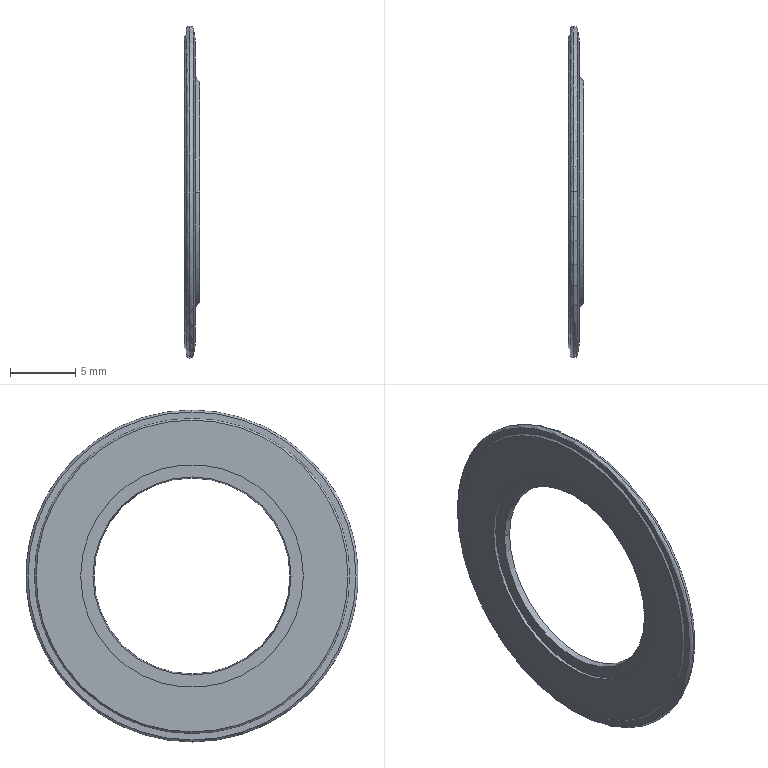Part | SolidWorks | features BaseBody 1 | 1 solid | 23 faces | box 1.155 x 25.353 x 25.353 mm | volume 176.021 mm3 | cone 8 | cylinder 6 | plane 5 | torus 4 | commonest cylinder face diameters 17 x4 23.324 x2
STEP:
#1=CARTESIAN_POINT('',(0.456,0.,12.676));
#2=VERTEX_POINT('',#1);
#3=CARTESIAN_POINT('',(0.456,0.,-12.676));
#4=VERTEX_POINT('',#3);
#5=CARTESIAN_POINT('',(0.456,0.,0.));
#6=DIRECTION('',(1.,0.,0.));
#7=DIRECTION('',(0.,0.,-1.));
#8=AXIS2_PLACEMENT_3D('',#5,#6,#7);
#9=CIRCLE('',#8,12.676);
#10=EDGE_CURVE('',#2,#4,#9,.T.);
#11=ORIENTED_EDGE('',*,*,#10,.T.);
#12=CARTESIAN_POINT('',(0.7554,0.,-12.425));
#13=VERTEX_POINT('',#12);
#14=CARTESIAN_POINT('',(0.456,0.,-12.372));
#15=DIRECTION('',(0.,-1.,0.));
#16=DIRECTION('',(0.,0.,-1.));
#17=AXIS2_PLACEMENT_3D('',#14,#15,#16);
#18=CIRCLE('',#17,0.304);
#19=EDGE_CURVE('',#4,#13,#18,.T.);
#20=ORIENTED_EDGE('',*,*,#19,.T.);
#21=CARTESIAN_POINT('',(0.7554,-12.425,0.));
#22=VERTEX_POINT('',#21);
#23=CARTESIAN_POINT('',(0.7554,0.,0.));
#24=DIRECTION('',(1.,0.,0.));
#25=DIRECTION('',(0.,1.,0.));
#26=AXIS2_PLACEMENT_3D('',#23,#24,#25);
#27=CIRCLE('',#26,12.425);
#28=EDGE_CURVE('',#22,#13,#27,.T.);
#29=ORIENTED_EDGE('',*,*,#28,.F.);
#30=CARTESIAN_POINT('',(0.7554,0.,12.425));
#31=VERTEX_POINT('',#30);
#32=CARTESIAN_POINT('',(0.7554,0.,0.));
#33=DIRECTION('',(1.,0.,0.));
#34=DIRECTION('',(0.,1.,0.));
#35=AXIS2_PLACEMENT_3D('',#32,#33,#34);
#36=CIRCLE('',#35,12.425);
#37=EDGE_CURVE('',#31,#22,#36,.T.);
#38=ORIENTED_EDGE('',*,*,#37,.F.);
#39=CARTESIAN_POINT('',(0.456,0.,12.372));
#40=DIRECTION('',(0.,-1.,0.));
#41=DIRECTION('',(0.,0.,1.));
#42=AXIS2_PLACEMENT_3D('',#39,#40,#41);
#43=CIRCLE('',#42,0.304);
#44=EDGE_CURVE('',#31,#2,#43,.T.);
#45=ORIENTED_EDGE('',*,*,#44,.T.);
#46=EDGE_LOOP('',(#11,#20,#29,#38,#45));
#47=FACE_OUTER_BOUND('',#46,.T.);
#48=CARTESIAN_POINT('',(0.456,0.,0.));
#49=DIRECTION('',(1.,0.,0.));
#50=DIRECTION('',(0.,0.,-1.));
#51=AXIS2_PLACEMENT_3D('',#48,#49,#50);
#52=TOROIDAL_SURFACE('',#51,12.372,0.304);
#53=ADVANCED_FACE('',(#47),#52,.T.);
#54=CARTESIAN_POINT('',(0.1927,12.038,0.));
#55=VERTEX_POINT('',#54);
#56=CARTESIAN_POINT('',(0.1927,-12.038,0.));
#57=VERTEX_POINT('',#56);
#58=CARTESIAN_POINT('',(0.1927,0.,0.));
#59=DIRECTION('',(1.,0.,0.));
#60=DIRECTION('',(0.,1.,0.));
#61=AXIS2_PLACEMENT_3D('',#58,#59,#60);
#62=CIRCLE('',#61,12.038);
#63=EDGE_CURVE('',#55,#57,#62,.T.);
#64=ORIENTED_EDGE('',*,*,#63,.T.);
#65=CARTESIAN_POINT('',(0.1927,0.,0.));
#66=DIRECTION('',(1.,0.,0.));
#67=DIRECTION('',(0.,1.,0.));
#68=AXIS2_PLACEMENT_3D('',#65,#66,#67);
#69=CIRCLE('',#68,12.038);
#70=EDGE_CURVE('',#57,#55,#69,.T.);
#71=ORIENTED_EDGE('',*,*,#70,.T.);
#72=EDGE_LOOP('',(#64,#71));
#73=FACE_BOUND('',#72,.T.);
#74=CARTESIAN_POINT('',(0.1927,0.,-12.524));
#75=VERTEX_POINT('',#74);
#76=CARTESIAN_POINT('',(0.1927,0.,12.524));
#77=VERTEX_POINT('',#76);
#78=CARTESIAN_POINT('',(0.1927,0.,0.));
#79=DIRECTION('',(1.,0.,0.));
#80=DIRECTION('',(0.,1.,0.));
#81=AXIS2_PLACEMENT_3D('',#78,#79,#80);
#82=CIRCLE('',#81,12.524);
#83=EDGE_CURVE('',#75,#77,#82,.T.);
#84=ORIENTED_EDGE('',*,*,#83,.F.);
#85=CARTESIAN_POINT('',(0.1927,0.,0.));
#86=DIRECTION('',(1.,0.,0.));
#87=DIRECTION('',(0.,1.,0.));
#88=AXIS2_PLACEMENT_3D('',#85,#86,#87);
#89=CIRCLE('',#88,12.524);
#90=EDGE_CURVE('',#77,#75,#89,.T.);
#91=ORIENTED_EDGE('',*,*,#90,.F.);
#92=EDGE_LOOP('',(#84,#91));
#93=FACE_OUTER_BOUND('',#92,.T.);
#94=CARTESIAN_POINT('',(0.1927,12.281,0.));
#95=DIRECTION('',(-1.,0.,0.));
#96=DIRECTION('',(0.,1.,0.));
#97=AXIS2_PLACEMENT_3D('',#94,#95,#96);
#98=PLANE('',#97);
#99=ADVANCED_FACE('',(#73,#93),#98,.T.);
#100=CARTESIAN_POINT('',(0.0608,11.906,0.));
#101=VERTEX_POINT('',#100);
#102=CARTESIAN_POINT('',(0.1268,11.972,0.));
#103=DIRECTION('',(0.7071,0.7071,0.));
#104=VECTOR('',#103,1000.);
#105=LINE('',#102,#104);
#106=EDGE_CURVE('',#101,#55,#105,.T.);
#107=ORIENTED_EDGE('',*,*,#106,.T.);
#108=ORIENTED_EDGE('',*,*,#70,.F.);
#109=CARTESIAN_POINT('',(0.0608,-11.906,0.));
#110=VERTEX_POINT('',#109);
#111=CARTESIAN_POINT('',(0.1268,-11.972,0.));
#112=DIRECTION('',(-0.7071,0.7071,0.));
#113=VECTOR('',#112,1000.);
#114=LINE('',#111,#113);
#115=EDGE_CURVE('',#57,#110,#114,.T.);
#116=ORIENTED_EDGE('',*,*,#115,.T.);
#117=CARTESIAN_POINT('',(0.0608,0.,0.));
#118=DIRECTION('',(1.,0.,0.));
#119=DIRECTION('',(0.,1.,0.));
#120=AXIS2_PLACEMENT_3D('',#117,#118,#119);
#121=CIRCLE('',#120,11.906);
#122=EDGE_CURVE('',#110,#101,#121,.T.);
#123=ORIENTED_EDGE('',*,*,#122,.T.);
#124=EDGE_LOOP('',(#107,#108,#116,#123));
#125=FACE_OUTER_BOUND('',#124,.T.);
#126=CARTESIAN_POINT('',(0.1268,0.,0.));
#127=DIRECTION('',(1.,0.,0.));
#128=DIRECTION('',(0.,1.,0.));
#129=AXIS2_PLACEMENT_3D('',#126,#127,#128);
#130=CONICAL_SURFACE('',#129,11.972,0.7854);
#131=ADVANCED_FACE('',(#125),#130,.T.);
#132=CARTESIAN_POINT('',(0.0608,8.5,0.));
#133=VERTEX_POINT('',#132);
#134=CARTESIAN_POINT('',(0.0608,-8.5,0.));
#135=VERTEX_POINT('',#134);
#136=CARTESIAN_POINT('',(0.0608,0.,0.));
#137=DIRECTION('',(1.,0.,0.));
#138=DIRECTION('',(0.,1.,0.));
#139=AXIS2_PLACEMENT_3D('',#136,#137,#138);
#140=CIRCLE('',#139,8.5);
#141=EDGE_CURVE('',#133,#135,#140,.T.);
#142=ORIENTED_EDGE('',*,*,#141,.T.);
#143=CARTESIAN_POINT('',(0.0608,0.,0.));
#144=DIRECTION('',(1.,0.,0.));
#145=DIRECTION('',(0.,1.,0.));
#146=AXIS2_PLACEMENT_3D('',#143,#144,#145);
#147=CIRCLE('',#146,8.5);
#148=EDGE_CURVE('',#135,#133,#147,.T.);
#149=ORIENTED_EDGE('',*,*,#148,.T.);
#150=EDGE_LOOP('',(#142,#149));
#151=FACE_BOUND('',#150,.T.);
#152=CARTESIAN_POINT('',(0.0608,0.,0.));
#153=DIRECTION('',(1.,0.,0.));
#154=DIRECTION('',(0.,1.,0.));
#155=AXIS2_PLACEMENT_3D('',#152,#153,#154);
#156=CIRCLE('',#155,11.906);
#157=EDGE_CURVE('',#101,#110,#156,.T.);
#158=ORIENTED_EDGE('',*,*,#157,.F.);
#159=ORIENTED_EDGE('',*,*,#122,.F.);
#160=EDGE_LOOP('',(#158,#159));
#161=FACE_OUTER_BOUND('',#160,.T.);
#162=CARTESIAN_POINT('',(0.0608,10.203,0.));
#163=DIRECTION('',(-1.,0.,0.));
#164=DIRECTION('',(0.,0.,1.));
#165=AXIS2_PLACEMENT_3D('',#162,#163,#164);
#166=PLANE('',#165);
#167=ADVANCED_FACE('',(#151,#161),#166,.T.);
#168=CARTESIAN_POINT('',(0.2888,8.5,0.));
#169=VERTEX_POINT('',#168);
#170=CARTESIAN_POINT('',(0.1748,8.5,0.));
#171=DIRECTION('',(1.,0.,0.));
#172=VECTOR('',#171,1000.);
#173=LINE('',#170,#172);
#174=EDGE_CURVE('',#133,#169,#173,.T.);
#175=ORIENTED_EDGE('',*,*,#174,.T.);
#176=CARTESIAN_POINT('',(0.2888,-8.5,0.));
#177=VERTEX_POINT('',#176);
#178=CARTESIAN_POINT('',(0.2888,0.,0.));
#179=DIRECTION('',(1.,0.,0.));
#180=DIRECTION('',(0.,1.,0.));
#181=AXIS2_PLACEMENT_3D('',#178,#179,#180);
#182=CIRCLE('',#181,8.5);
#183=EDGE_CURVE('',#169,#177,#182,.T.);
#184=ORIENTED_EDGE('',*,*,#183,.T.);
#185=CARTESIAN_POINT('',(0.1748,-8.5,0.));
#186=DIRECTION('',(-1.,0.,0.));
#187=VECTOR('',#186,1000.);
#188=LINE('',#185,#187);
#189=EDGE_CURVE('',#177,#135,#188,.T.);
#190=ORIENTED_EDGE('',*,*,#189,.T.);
#191=ORIENTED_EDGE('',*,*,#141,.F.);
#192=EDGE_LOOP('',(#175,#184,#190,#191));
#193=FACE_OUTER_BOUND('',#192,.T.);
#194=CARTESIAN_POINT('',(0.1748,0.,0.));
#195=DIRECTION('',(1.,0.,0.));
#196=DIRECTION('',(0.,1.,0.));
#197=AXIS2_PLACEMENT_3D('',#194,#195,#196);
#198=CYLINDRICAL_SURFACE('',#197,8.5);
#199=ADVANCED_FACE('',(#193),#198,.F.);
#200=CARTESIAN_POINT('',(0.2888,7.565,0.));
#201=VERTEX_POINT('',#200);
#202=CARTESIAN_POINT('',(0.2888,-7.565,0.));
#203=VERTEX_POINT('',#202);
#204=CARTESIAN_POINT('',(0.2888,0.,0.));
#205=DIRECTION('',(1.,0.,0.));
#206=DIRECTION('',(0.,1.,0.));
#207=AXIS2_PLACEMENT_3D('',#204,#205,#206);
#208=CIRCLE('',#207,7.565);
#209=EDGE_CURVE('',#201,#203,#208,.T.);
#210=ORIENTED_EDGE('',*,*,#209,.T.);
#211=CARTESIAN_POINT('',(0.2888,0.,0.));
#212=DIRECTION('',(1.,0.,0.));
#213=DIRECTION('',(0.,1.,0.));
#214=AXIS2_PLACEMENT_3D('',#211,#212,#213);
#215=CIRCLE('',#214,7.565);
#216=EDGE_CURVE('',#203,#201,#215,.T.);
#217=ORIENTED_EDGE('',*,*,#216,.T.);
#218=EDGE_LOOP('',(#210,#217));
#219=FACE_BOUND('',#218,.T.);
#220=ORIENTED_EDGE('',*,*,#183,.F.);
#221=CARTESIAN_POINT('',(0.2888,0.,0.));
#222=DIRECTION('',(1.,0.,0.));
#223=DIRECTION('',(0.,1.,0.));
#224=AXIS2_PLACEMENT_3D('',#221,#222,#223);
#225=CIRCLE('',#224,8.5);
#226=EDGE_CURVE('',#177,#169,#225,.T.);
#227=ORIENTED_EDGE('',*,*,#226,.F.);
#228=EDGE_LOOP('',(#220,#227));
#229=FACE_OUTER_BOUND('',#228,.T.);
#230=CARTESIAN_POINT('',(0.2888,8.033,0.));
#231=DIRECTION('',(-1.,0.,0.));
#232=DIRECTION('',(0.,1.,0.));
#233=AXIS2_PLACEMENT_3D('',#230,#231,#232);
#234=PLANE('',#233);
#235=ADVANCED_FACE('',(#219,#229),#234,.T.);
#236=CARTESIAN_POINT('',(0.76,7.482,0.));
#237=VERTEX_POINT('',#236);
#238=CARTESIAN_POINT('',(0.5244,7.524,0.));
#239=DIRECTION('',(0.9848,-0.1736,0.));
#240=VECTOR('',#239,1000.);
#241=LINE('',#238,#240);
#242=EDGE_CURVE('',#201,#237,#241,.T.);
#243=ORIENTED_EDGE('',*,*,#242,.T.);
#244=CARTESIAN_POINT('',(0.76,-7.482,0.));
#245=VERTEX_POINT('',#244);
#246=CARTESIAN_POINT('',(0.76,0.,0.));
#247=DIRECTION('',(1.,0.,0.));
#248=DIRECTION('',(0.,1.,0.));
#249=AXIS2_PLACEMENT_3D('',#246,#247,#248);
#250=CIRCLE('',#249,7.482);
#251=EDGE_CURVE('',#237,#245,#250,.T.);
#252=ORIENTED_EDGE('',*,*,#251,.T.);
#253=CARTESIAN_POINT('',(0.5244,-7.524,0.));
#254=DIRECTION('',(-0.9848,-0.1736,0.));
#255=VECTOR('',#254,1000.);
#256=LINE('',#253,#255);
#257=EDGE_CURVE('',#245,#203,#256,.T.);
#258=ORIENTED_EDGE('',*,*,#257,.T.);
#259=ORIENTED_EDGE('',*,*,#209,.F.);
#260=EDGE_LOOP('',(#243,#252,#258,#259));
#261=FACE_OUTER_BOUND('',#260,.T.);
#262=CARTESIAN_POINT('',(0.5244,0.,0.));
#263=DIRECTION('',(-1.,0.,0.));
#264=DIRECTION('',(0.,1.,0.));
#265=AXIS2_PLACEMENT_3D('',#262,#263,#264);
#266=CONICAL_SURFACE('',#265,7.524,0.1745);
#267=ADVANCED_FACE('',(#261),#266,.F.);
#268=ORIENTED_EDGE('',*,*,#251,.F.);
#269=CARTESIAN_POINT('',(0.76,0.,0.));
#270=DIRECTION('',(1.,0.,0.));
#271=DIRECTION('',(0.,1.,0.));
#272=AXIS2_PLACEMENT_3D('',#269,#270,#271);
#273=CIRCLE('',#272,7.482);
#274=EDGE_CURVE('',#245,#237,#273,.T.);
#275=ORIENTED_EDGE('',*,*,#274,.F.);
#276=EDGE_LOOP('',(#268,#275));
#277=FACE_BOUND('',#276,.T.);
#278=CARTESIAN_POINT('',(0.76,8.5,0.));
#279=VERTEX_POINT('',#278);
#280=CARTESIAN_POINT('',(0.76,-8.5,0.));
#281=VERTEX_POINT('',#280);
#282=CARTESIAN_POINT('',(0.76,0.,0.));
#283=DIRECTION('',(1.,0.,0.));
#284=DIRECTION('',(0.,1.,0.));
#285=AXIS2_PLACEMENT_3D('',#282,#283,#284);
#286=CIRCLE('',#285,8.5);
#287=EDGE_CURVE('',#279,#281,#286,.T.);
#288=ORIENTED_EDGE('',*,*,#287,.T.);
#289=CARTESIAN_POINT('',(0.76,0.,0.));
#290=DIRECTION('',(1.,0.,0.));
#291=DIRECTION('',(0.,1.,0.));
#292=AXIS2_PLACEMENT_3D('',#289,#290,#291);
#293=CIRCLE('',#292,8.5);
#294=EDGE_CURVE('',#281,#279,#293,.T.);
#295=ORIENTED_EDGE('',*,*,#294,.T.);
#296=EDGE_LOOP('',(#288,#295));
#297=FACE_OUTER_BOUND('',#296,.T.);
#298=CARTESIAN_POINT('',(0.76,7.991,0.));
#299=DIRECTION('',(1.,0.,0.));
#300=DIRECTION('',(0.,1.,0.));
#301=AXIS2_PLACEMENT_3D('',#298,#299,#300);
#302=PLANE('',#301);
#303=ADVANCED_FACE('',(#277,#297),#302,.T.);
#304=CARTESIAN_POINT('',(1.216,8.5,0.));
#305=VERTEX_POINT('',#304);
#306=CARTESIAN_POINT('',(0.988,8.5,0.));
#307=DIRECTION('',(1.,0.,0.));
#308=VECTOR('',#307,1000.);
#309=LINE('',#306,#308);
#310=EDGE_CURVE('',#279,#305,#309,.T.);
#311=ORIENTED_EDGE('',*,*,#310,.T.);
#312=CARTESIAN_POINT('',(1.216,-8.5,0.));
#313=VERTEX_POINT('',#312);
#314=CARTESIAN_POINT('',(1.216,0.,0.));
#315=DIRECTION('',(1.,0.,0.));
#316=DIRECTION('',(0.,1.,0.));
#317=AXIS2_PLACEMENT_3D('',#314,#315,#316);
#318=CIRCLE('',#317,8.5);
#319=EDGE_CURVE('',#305,#313,#318,.T.);
#320=ORIENTED_EDGE('',*,*,#319,.T.);
#321=CARTESIAN_POINT('',(0.988,-8.5,0.));
#322=DIRECTION('',(-1.,0.,0.));
#323=VECTOR('',#322,1000.);
#324=LINE('',#321,#323);
#325=EDGE_CURVE('',#313,#281,#324,.T.);
#326=ORIENTED_EDGE('',*,*,#325,.T.);
#327=ORIENTED_EDGE('',*,*,#287,.F.);
#328=EDGE_LOOP('',(#311,#320,#326,#327));
#329=FACE_OUTER_BOUND('',#328,.T.);
#330=CARTESIAN_POINT('',(0.988,0.,0.));
#331=DIRECTION('',(1.,0.,0.));
#332=DIRECTION('',(0.,1.,0.));
#333=AXIS2_PLACEMENT_3D('',#330,#331,#332);
#334=CYLINDRICAL_SURFACE('',#333,8.5);
#335=ADVANCED_FACE('',(#329),#334,.F.);
#336=CARTESIAN_POINT('',(0.5168,9.199,0.));
#337=VERTEX_POINT('',#336);
#338=CARTESIAN_POINT('',(0.8664,8.85,0.));
#339=DIRECTION('',(0.7071,-0.7071,0.));
#340=VECTOR('',#339,1000.);
#341=LINE('',#338,#340);
#342=EDGE_CURVE('',#337,#305,#341,.T.);
#343=ORIENTED_EDGE('',*,*,#342,.T.);
#344=CARTESIAN_POINT('',(1.216,0.,0.));
#345=DIRECTION('',(1.,0.,0.));
#346=DIRECTION('',(0.,1.,0.));
#347=AXIS2_PLACEMENT_3D('',#344,#345,#346);
#348=CIRCLE('',#347,8.5);
#349=EDGE_CURVE('',#313,#305,#348,.T.);
#350=ORIENTED_EDGE('',*,*,#349,.F.);
#351=CARTESIAN_POINT('',(0.5168,-9.199,0.));
#352=VERTEX_POINT('',#351);
#353=CARTESIAN_POINT('',(0.8664,-8.85,0.));
#354=DIRECTION('',(-0.7071,-0.7071,0.));
#355=VECTOR('',#354,1000.);
#356=LINE('',#353,#355);
#357=EDGE_CURVE('',#313,#352,#356,.T.);
#358=ORIENTED_EDGE('',*,*,#357,.T.);
#359=CARTESIAN_POINT('',(0.5168,0.,0.));
#360=DIRECTION('',(1.,0.,0.));
#361=DIRECTION('',(0.,1.,0.));
#362=AXIS2_PLACEMENT_3D('',#359,#360,#361);
#363=CIRCLE('',#362,9.199);
#364=EDGE_CURVE('',#352,#337,#363,.T.);
#365=ORIENTED_EDGE('',*,*,#364,.T.);
#366=EDGE_LOOP('',(#343,#350,#358,#365));
#367=FACE_OUTER_BOUND('',#366,.T.);
#368=CARTESIAN_POINT('',(0.8664,0.,0.));
#369=DIRECTION('',(-1.,0.,0.));
#370=DIRECTION('',(0.,1.,0.));
#371=AXIS2_PLACEMENT_3D('',#368,#369,#370);
#372=CONICAL_SURFACE('',#371,8.85,0.7854);
#373=ADVANCED_FACE('',(#367),#372,.T.);
#374=CARTESIAN_POINT('',(0.5168,0.,0.));
#375=DIRECTION('',(1.,0.,0.));
#376=DIRECTION('',(0.,1.,0.));
#377=AXIS2_PLACEMENT_3D('',#374,#375,#376);
#378=CIRCLE('',#377,9.199);
#379=EDGE_CURVE('',#337,#352,#378,.T.);
#380=ORIENTED_EDGE('',*,*,#379,.F.);
#381=ORIENTED_EDGE('',*,*,#364,.F.);
#382=EDGE_LOOP('',(#380,#381));
#383=FACE_BOUND('',#382,.T.);
#384=CARTESIAN_POINT('',(0.5168,11.662,0.));
#385=VERTEX_POINT('',#384);
#386=CARTESIAN_POINT('',(0.5168,-11.662,0.));
#387=VERTEX_POINT('',#386);
#388=CARTESIAN_POINT('',(0.5168,0.,0.));
#389=DIRECTION('',(1.,0.,0.));
#390=DIRECTION('',(0.,1.,0.));
#391=AXIS2_PLACEMENT_3D('',#388,#389,#390);
#392=CIRCLE('',#391,11.662);
#393=EDGE_CURVE('',#385,#387,#392,.T.);
#394=ORIENTED_EDGE('',*,*,#393,.T.);
#395=CARTESIAN_POINT('',(0.5168,0.,0.));
#396=DIRECTION('',(1.,0.,0.));
#397=DIRECTION('',(0.,1.,0.));
#398=AXIS2_PLACEMENT_3D('',#395,#396,#397);
#399=CIRCLE('',#398,11.662);
#400=EDGE_CURVE('',#387,#385,#399,.T.);
#401=ORIENTED_EDGE('',*,*,#400,.T.);
#402=EDGE_LOOP('',(#394,#401));
#403=FACE_OUTER_BOUND('',#402,.T.);
#404=CARTESIAN_POINT('',(0.5168,10.431,0.));
#405=DIRECTION('',(1.,0.,0.));
#406=DIRECTION('',(0.,1.,0.));
#407=AXIS2_PLACEMENT_3D('',#404,#405,#406);
#408=PLANE('',#407);
#409=ADVANCED_FACE('',(#383,#403),#408,.T.);
#410=CARTESIAN_POINT('',(0.8899,11.662,0.));
#411=VERTEX_POINT('',#410);
#412=CARTESIAN_POINT('',(0.7034,11.662,0.));
#413=DIRECTION('',(1.,0.,0.));
#414=VECTOR('',#413,1000.);
#415=LINE('',#412,#414);
#416=EDGE_CURVE('',#385,#411,#415,.T.);
#417=ORIENTED_EDGE('',*,*,#416,.T.);
#418=CARTESIAN_POINT('',(0.8899,-11.662,0.));
#419=VERTEX_POINT('',#418);
#420=CARTESIAN_POINT('',(0.8899,0.,0.));
#421=DIRECTION('',(1.,0.,0.));
#422=DIRECTION('',(0.,1.,0.));
#423=AXIS2_PLACEMENT_3D('',#420,#421,#422);
#424=CIRCLE('',#423,11.662);
#425=EDGE_CURVE('',#411,#419,#424,.T.);
#426=ORIENTED_EDGE('',*,*,#425,.T.);
#427=CARTESIAN_POINT('',(0.7034,-11.662,0.));
#428=DIRECTION('',(-1.,0.,0.));
#429=VECTOR('',#428,1000.);
#430=LINE('',#427,#429);
#431=EDGE_CURVE('',#419,#387,#430,.T.);
#432=ORIENTED_EDGE('',*,*,#431,.T.);
#433=ORIENTED_EDGE('',*,*,#393,.F.);
#434=EDGE_LOOP('',(#417,#426,#432,#433));
#435=FACE_OUTER_BOUND('',#434,.T.);
#436=CARTESIAN_POINT('',(0.7034,0.,0.));
#437=DIRECTION('',(1.,0.,0.));
#438=DIRECTION('',(0.,1.,0.));
#439=AXIS2_PLACEMENT_3D('',#436,#437,#438);
#440=CYLINDRICAL_SURFACE('',#439,11.662);
#441=ADVANCED_FACE('',(#435),#440,.F.);
#442=CARTESIAN_POINT('',(0.7554,12.425,0.));
#443=VERTEX_POINT('',#442);
#444=CARTESIAN_POINT('',(0.8227,12.044,0.));
#445=DIRECTION('',(0.1736,-0.9848,0.));
#446=VECTOR('',#445,1000.);
#447=LINE('',#444,#446);
#448=EDGE_CURVE('',#443,#411,#447,.T.);
#449=ORIENTED_EDGE('',*,*,#448,.T.);
#450=CARTESIAN_POINT('',(0.8899,0.,0.));
#451=DIRECTION('',(1.,0.,0.));
#452=DIRECTION('',(0.,1.,0.));
#453=AXIS2_PLACEMENT_3D('',#450,#451,#452);
#454=CIRCLE('',#453,11.662);
#455=EDGE_CURVE('',#419,#411,#454,.T.);
#456=ORIENTED_EDGE('',*,*,#455,.F.);
#457=CARTESIAN_POINT('',(0.8227,-12.044,0.));
#458=DIRECTION('',(-0.1736,-0.9848,0.));
#459=VECTOR('',#458,1000.);
#460=LINE('',#457,#459);
#461=EDGE_CURVE('',#419,#22,#460,.T.);
#462=ORIENTED_EDGE('',*,*,#461,.T.);
#463=ORIENTED_EDGE('',*,*,#28,.T.);
#464=CARTESIAN_POINT('',(0.7554,0.,0.));
#465=DIRECTION('',(1.,0.,0.));
#466=DIRECTION('',(0.,1.,0.));
#467=AXIS2_PLACEMENT_3D('',#464,#465,#466);
#468=CIRCLE('',#467,12.425);
#469=EDGE_CURVE('',#13,#443,#468,.T.);
#470=ORIENTED_EDGE('',*,*,#469,.T.);
#471=EDGE_LOOP('',(#449,#456,#462,#463,#470));
#472=FACE_OUTER_BOUND('',#471,.T.);
#473=CARTESIAN_POINT('',(0.8227,0.,0.));
#474=DIRECTION('',(-1.,0.,0.));
#475=DIRECTION('',(0.,1.,0.));
#476=AXIS2_PLACEMENT_3D('',#473,#474,#475);
#477=CONICAL_SURFACE('',#476,12.044,1.396);
#478=ADVANCED_FACE('',(#472),#477,.T.);
#479=ORIENTED_EDGE('',*,*,#448,.F.);
#480=CARTESIAN_POINT('',(0.7554,0.,0.));
#481=DIRECTION('',(1.,0.,0.));
#482=DIRECTION('',(0.,1.,0.));
#483=AXIS2_PLACEMENT_3D('',#480,#481,#482);
#484=CIRCLE('',#483,12.425);
#485=EDGE_CURVE('',#443,#31,#484,.T.);
#486=ORIENTED_EDGE('',*,*,#485,.T.);
#487=ORIENTED_EDGE('',*,*,#37,.T.);
#488=ORIENTED_EDGE('',*,*,#461,.F.);
#489=ORIENTED_EDGE('',*,*,#425,.F.);
#490=EDGE_LOOP('',(#479,#486,#487,#488,#489));
#491=FACE_OUTER_BOUND('',#490,.T.);
#492=CARTESIAN_POINT('',(0.8227,0.,0.));
#493=DIRECTION('',(-1.,0.,0.));
#494=DIRECTION('',(0.,1.,0.));
#495=AXIS2_PLACEMENT_3D('',#492,#493,#494);
#496=CONICAL_SURFACE('',#495,12.044,1.396);
#497=ADVANCED_FACE('',(#491),#496,.T.);
#498=ORIENTED_EDGE('',*,*,#416,.F.);
#499=ORIENTED_EDGE('',*,*,#400,.F.);
#500=ORIENTED_EDGE('',*,*,#431,.F.);
#501=ORIENTED_EDGE('',*,*,#455,.T.);
#502=EDGE_LOOP('',(#498,#499,#500,#501));
#503=FACE_OUTER_BOUND('',#502,.T.);
#504=CARTESIAN_POINT('',(0.7034,0.,0.));
#505=DIRECTION('',(1.,0.,0.));
#506=DIRECTION('',(0.,1.,0.));
#507=AXIS2_PLACEMENT_3D('',#504,#505,#506);
#508=CYLINDRICAL_SURFACE('',#507,11.662);
#509=ADVANCED_FACE('',(#503),#508,.F.);
#510=ORIENTED_EDGE('',*,*,#342,.F.);
#511=ORIENTED_EDGE('',*,*,#379,.T.);
#512=ORIENTED_EDGE('',*,*,#357,.F.);
#513=ORIENTED_EDGE('',*,*,#319,.F.);
#514=EDGE_LOOP('',(#510,#511,#512,#513));
#515=FACE_OUTER_BOUND('',#514,.T.);
#516=CARTESIAN_POINT('',(0.8664,0.,0.));
#517=DIRECTION('',(-1.,0.,0.));
#518=DIRECTION('',(0.,1.,0.));
#519=AXIS2_PLACEMENT_3D('',#516,#517,#518);
#520=CONICAL_SURFACE('',#519,8.85,0.7854);
#521=ADVANCED_FACE('',(#515),#520,.T.);
#522=ORIENTED_EDGE('',*,*,#310,.F.);
#523=ORIENTED_EDGE('',*,*,#294,.F.);
#524=ORIENTED_EDGE('',*,*,#325,.F.);
#525=ORIENTED_EDGE('',*,*,#349,.T.);
#526=EDGE_LOOP('',(#522,#523,#524,#525));
#527=FACE_OUTER_BOUND('',#526,.T.);
#528=CARTESIAN_POINT('',(0.988,0.,0.));
#529=DIRECTION('',(1.,0.,0.));
#530=DIRECTION('',(0.,1.,0.));
#531=AXIS2_PLACEMENT_3D('',#528,#529,#530);
#532=CYLINDRICAL_SURFACE('',#531,8.5);
#533=ADVANCED_FACE('',(#527),#532,.F.);
#534=ORIENTED_EDGE('',*,*,#242,.F.);
#535=ORIENTED_EDGE('',*,*,#216,.F.);
#536=ORIENTED_EDGE('',*,*,#257,.F.);
#537=ORIENTED_EDGE('',*,*,#274,.T.);
#538=EDGE_LOOP('',(#534,#535,#536,#537));
#539=FACE_OUTER_BOUND('',#538,.T.);
#540=CARTESIAN_POINT('',(0.5244,0.,0.));
#541=DIRECTION('',(-1.,0.,0.));
#542=DIRECTION('',(0.,1.,0.));
#543=AXIS2_PLACEMENT_3D('',#540,#541,#542);
#544=CONICAL_SURFACE('',#543,7.524,0.1745);
#545=ADVANCED_FACE('',(#539),#544,.F.);
#546=ORIENTED_EDGE('',*,*,#174,.F.);
#547=ORIENTED_EDGE('',*,*,#148,.F.);
#548=ORIENTED_EDGE('',*,*,#189,.F.);
#549=ORIENTED_EDGE('',*,*,#226,.T.);
#550=EDGE_LOOP('',(#546,#547,#548,#549));
#551=FACE_OUTER_BOUND('',#550,.T.);
#552=CARTESIAN_POINT('',(0.1748,0.,0.));
#553=DIRECTION('',(1.,0.,0.));
#554=DIRECTION('',(0.,1.,0.));
#555=AXIS2_PLACEMENT_3D('',#552,#553,#554);
#556=CYLINDRICAL_SURFACE('',#555,8.5);
#557=ADVANCED_FACE('',(#551),#556,.F.);
#558=ORIENTED_EDGE('',*,*,#106,.F.);
#559=ORIENTED_EDGE('',*,*,#157,.T.);
#560=ORIENTED_EDGE('',*,*,#115,.F.);
#561=ORIENTED_EDGE('',*,*,#63,.F.);
#562=EDGE_LOOP('',(#558,#559,#560,#561));
#563=FACE_OUTER_BOUND('',#562,.T.);
#564=CARTESIAN_POINT('',(0.1268,0.,0.));
#565=DIRECTION('',(1.,0.,0.));
#566=DIRECTION('',(0.,1.,0.));
#567=AXIS2_PLACEMENT_3D('',#564,#565,#566);
#568=CONICAL_SURFACE('',#567,11.972,0.7854);
#569=ADVANCED_FACE('',(#563),#568,.T.);
#570=CARTESIAN_POINT('',(0.456,0.,0.));
#571=DIRECTION('',(1.,0.,0.));
#572=DIRECTION('',(0.,0.,-1.));
#573=AXIS2_PLACEMENT_3D('',#570,#571,#572);
#574=CIRCLE('',#573,12.676);
#575=EDGE_CURVE('',#4,#2,#574,.T.);
#576=ORIENTED_EDGE('',*,*,#575,.T.);
#577=ORIENTED_EDGE('',*,*,#44,.F.);
#578=ORIENTED_EDGE('',*,*,#485,.F.);
#579=ORIENTED_EDGE('',*,*,#469,.F.);
#580=ORIENTED_EDGE('',*,*,#19,.F.);
#581=EDGE_LOOP('',(#576,#577,#578,#579,#580));
#582=FACE_OUTER_BOUND('',#581,.T.);
#583=CARTESIAN_POINT('',(0.456,0.,0.));
#584=DIRECTION('',(1.,0.,0.));
#585=DIRECTION('',(0.,0.,-1.));
#586=AXIS2_PLACEMENT_3D('',#583,#584,#585);
#587=TOROIDAL_SURFACE('',#586,12.372,0.304);
#588=ADVANCED_FACE('',(#582),#587,.T.);
#589=ORIENTED_EDGE('',*,*,#575,.F.);
#590=CARTESIAN_POINT('',(0.456,0.,-12.372));
#591=DIRECTION('',(0.,-1.,0.));
#592=DIRECTION('',(0.,0.,-1.));
#593=AXIS2_PLACEMENT_3D('',#590,#591,#592);
#594=CIRCLE('',#593,0.304);
#595=EDGE_CURVE('',#75,#4,#594,.T.);
#596=ORIENTED_EDGE('',*,*,#595,.F.);
#597=ORIENTED_EDGE('',*,*,#83,.T.);
#598=CARTESIAN_POINT('',(0.456,0.,12.372));
#599=DIRECTION('',(0.,-1.,0.));
#600=DIRECTION('',(0.,0.,1.));
#601=AXIS2_PLACEMENT_3D('',#598,#599,#600);
#602=CIRCLE('',#601,0.304);
#603=EDGE_CURVE('',#2,#77,#602,.T.);
#604=ORIENTED_EDGE('',*,*,#603,.F.);
#605=EDGE_LOOP('',(#589,#596,#597,#604));
#606=FACE_OUTER_BOUND('',#605,.T.);
#607=CARTESIAN_POINT('',(0.456,0.,0.));
#608=DIRECTION('',(1.,0.,0.));
#609=DIRECTION('',(0.,0.,-1.));
#610=AXIS2_PLACEMENT_3D('',#607,#608,#609);
#611=TOROIDAL_SURFACE('',#610,12.372,0.304);
#612=ADVANCED_FACE('',(#606),#611,.T.);
#613=ORIENTED_EDGE('',*,*,#10,.F.);
#614=ORIENTED_EDGE('',*,*,#603,.T.);
#615=ORIENTED_EDGE('',*,*,#90,.T.);
#616=ORIENTED_EDGE('',*,*,#595,.T.);
#617=EDGE_LOOP('',(#613,#614,#615,#616));
#618=FACE_OUTER_BOUND('',#617,.T.);
#619=CARTESIAN_POINT('',(0.456,0.,0.));
#620=DIRECTION('',(1.,0.,0.));
#621=DIRECTION('',(0.,0.,-1.));
#622=AXIS2_PLACEMENT_3D('',#619,#620,#621);
#623=TOROIDAL_SURFACE('',#622,12.372,0.304);
#624=ADVANCED_FACE('',(#618),#623,.T.);
#625=CLOSED_SHELL('',(#53,#99,#131,#167,#199,#235,#267,#303,#335,#373,#409,#441,#478,#497,#509,#521,#533,#545,#557,#569,#588,#612,#624));
#626=MANIFOLD_SOLID_BREP('',#625);
#627=CARTESIAN_POINT('',(0.,0.,0.));
#628=DIRECTION('',(0.,0.,1.));
#629=DIRECTION('',(1.,0.,0.));
#630=AXIS2_PLACEMENT_3D('',#627,#628,#629);
#631=(LENGTH_UNIT()NAMED_UNIT(*)SI_UNIT(.MILLI.,.METRE.));
#632=UNCERTAINTY_MEASURE_WITH_UNIT(LENGTH_MEASURE(0.00001),#631,'','');
#633=(NAMED_UNIT(*)PLANE_ANGLE_UNIT()SI_UNIT($,.RADIAN.));
#634=(NAMED_UNIT(*)SI_UNIT($,.STERADIAN.)SOLID_ANGLE_UNIT());
#635=(GEOMETRIC_REPRESENTATION_CONTEXT(3)GLOBAL_UNCERTAINTY_ASSIGNED_CONTEXT((#632))GLOBAL_UNIT_ASSIGNED_CONTEXT((#631,#633,#634))REPRESENTATION_CONTEXT('',''));
#636=ADVANCED_BREP_SHAPE_REPRESENTATION('',(#626,#630),#635);